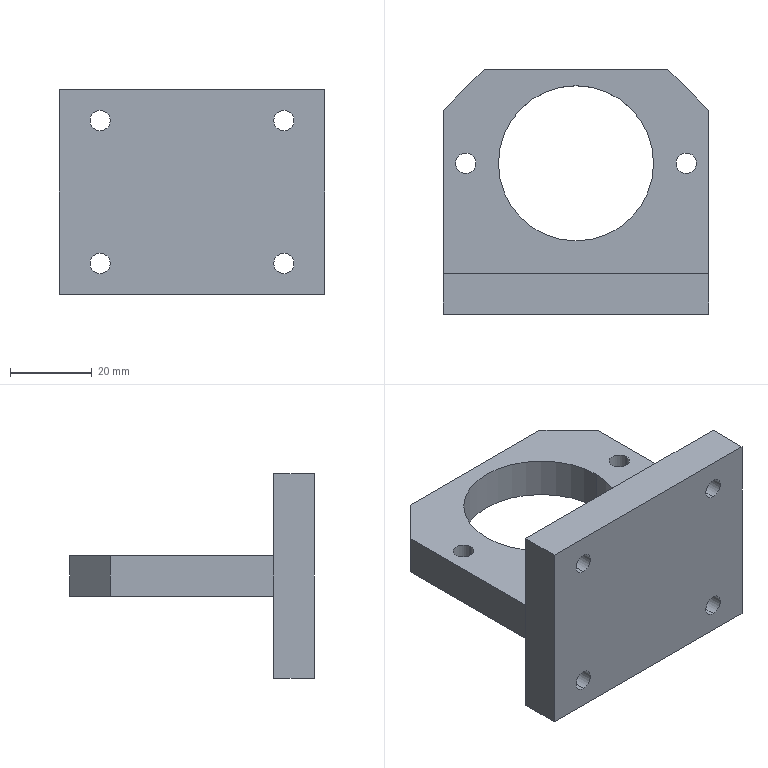Part | SolidWorks | features HoleWzd 2, ICE 2, Chamfer 1, Extrusion 1 | 2 solids | 28 faces | box 65 x 60 x 50 mm | volume 51481 mm3 | cylinder 14 | plane 14 | commonest cylinder face diameters 5 x12 38 x2
STEP:
#1=CARTESIAN_POINT('',(22.5,0.,15.));
#2=VERTEX_POINT('',#1);
#3=CARTESIAN_POINT('',(22.5,0.,20.));
#4=VERTEX_POINT('',#3);
#5=CARTESIAN_POINT('',(22.5,0.,17.5));
#6=DIRECTION('',(0.,1.,0.));
#7=DIRECTION('',(0.,0.,1.));
#8=AXIS2_PLACEMENT_3D('',#5,#6,#7);
#9=CIRCLE('',#8,2.5);
#10=EDGE_CURVE('',#2,#4,#9,.T.);
#11=ORIENTED_EDGE('',*,*,#10,.F.);
#12=CARTESIAN_POINT('',(22.5,10.,15.));
#13=VERTEX_POINT('',#12);
#14=CARTESIAN_POINT('',(22.5,10.,15.));
#15=DIRECTION('',(0.,1.,0.));
#16=VECTOR('',#15,1000.);
#17=LINE('',#14,#16);
#18=EDGE_CURVE('',#2,#13,#17,.T.);
#19=ORIENTED_EDGE('',*,*,#18,.T.);
#20=CARTESIAN_POINT('',(22.5,10.,20.));
#21=VERTEX_POINT('',#20);
#22=CARTESIAN_POINT('',(22.5,10.,17.5));
#23=DIRECTION('',(0.,1.,0.));
#24=DIRECTION('',(0.,0.,1.));
#25=AXIS2_PLACEMENT_3D('',#22,#23,#24);
#26=CIRCLE('',#25,2.5);
#27=EDGE_CURVE('',#13,#21,#26,.T.);
#28=ORIENTED_EDGE('',*,*,#27,.T.);
#29=CARTESIAN_POINT('',(22.5,10.,20.));
#30=DIRECTION('',(0.,1.,0.));
#31=VECTOR('',#30,1000.);
#32=LINE('',#29,#31);
#33=EDGE_CURVE('',#4,#21,#32,.T.);
#34=ORIENTED_EDGE('',*,*,#33,.F.);
#35=EDGE_LOOP('',(#11,#19,#28,#34));
#36=FACE_OUTER_BOUND('',#35,.T.);
#37=CARTESIAN_POINT('',(22.5,10.,17.5));
#38=DIRECTION('',(0.,1.,0.));
#39=DIRECTION('',(0.,0.,1.));
#40=AXIS2_PLACEMENT_3D('',#37,#38,#39);
#41=CYLINDRICAL_SURFACE('',#40,2.5);
#42=ADVANCED_FACE('',(#36),#41,.F.);
#43=CARTESIAN_POINT('',(-22.5,0.,-20.));
#44=VERTEX_POINT('',#43);
#45=CARTESIAN_POINT('',(-22.5,0.,-15.));
#46=VERTEX_POINT('',#45);
#47=CARTESIAN_POINT('',(-22.5,0.,-17.5));
#48=DIRECTION('',(0.,1.,0.));
#49=DIRECTION('',(0.,0.,1.));
#50=AXIS2_PLACEMENT_3D('',#47,#48,#49);
#51=CIRCLE('',#50,2.5);
#52=EDGE_CURVE('',#44,#46,#51,.T.);
#53=ORIENTED_EDGE('',*,*,#52,.F.);
#54=CARTESIAN_POINT('',(-22.5,10.,-20.));
#55=VERTEX_POINT('',#54);
#56=CARTESIAN_POINT('',(-22.5,10.,-20.));
#57=DIRECTION('',(0.,1.,0.));
#58=VECTOR('',#57,1000.);
#59=LINE('',#56,#58);
#60=EDGE_CURVE('',#44,#55,#59,.T.);
#61=ORIENTED_EDGE('',*,*,#60,.T.);
#62=CARTESIAN_POINT('',(-22.5,10.,-15.));
#63=VERTEX_POINT('',#62);
#64=CARTESIAN_POINT('',(-22.5,10.,-17.5));
#65=DIRECTION('',(0.,1.,0.));
#66=DIRECTION('',(0.,0.,1.));
#67=AXIS2_PLACEMENT_3D('',#64,#65,#66);
#68=CIRCLE('',#67,2.5);
#69=EDGE_CURVE('',#55,#63,#68,.T.);
#70=ORIENTED_EDGE('',*,*,#69,.T.);
#71=CARTESIAN_POINT('',(-22.5,10.,-15.));
#72=DIRECTION('',(0.,1.,0.));
#73=VECTOR('',#72,1000.);
#74=LINE('',#71,#73);
#75=EDGE_CURVE('',#46,#63,#74,.T.);
#76=ORIENTED_EDGE('',*,*,#75,.F.);
#77=EDGE_LOOP('',(#53,#61,#70,#76));
#78=FACE_OUTER_BOUND('',#77,.T.);
#79=CARTESIAN_POINT('',(-22.5,10.,-17.5));
#80=DIRECTION('',(0.,1.,0.));
#81=DIRECTION('',(0.,0.,1.));
#82=AXIS2_PLACEMENT_3D('',#79,#80,#81);
#83=CYLINDRICAL_SURFACE('',#82,2.5);
#84=ADVANCED_FACE('',(#78),#83,.F.);
#85=CARTESIAN_POINT('',(-22.5,0.,15.));
#86=VERTEX_POINT('',#85);
#87=CARTESIAN_POINT('',(-22.5,0.,20.));
#88=VERTEX_POINT('',#87);
#89=CARTESIAN_POINT('',(-22.5,0.,17.5));
#90=DIRECTION('',(0.,1.,0.));
#91=DIRECTION('',(0.,0.,1.));
#92=AXIS2_PLACEMENT_3D('',#89,#90,#91);
#93=CIRCLE('',#92,2.5);
#94=EDGE_CURVE('',#86,#88,#93,.T.);
#95=ORIENTED_EDGE('',*,*,#94,.F.);
#96=CARTESIAN_POINT('',(-22.5,10.,15.));
#97=VERTEX_POINT('',#96);
#98=CARTESIAN_POINT('',(-22.5,10.,15.));
#99=DIRECTION('',(0.,1.,0.));
#100=VECTOR('',#99,1000.);
#101=LINE('',#98,#100);
#102=EDGE_CURVE('',#86,#97,#101,.T.);
#103=ORIENTED_EDGE('',*,*,#102,.T.);
#104=CARTESIAN_POINT('',(-22.5,10.,20.));
#105=VERTEX_POINT('',#104);
#106=CARTESIAN_POINT('',(-22.5,10.,17.5));
#107=DIRECTION('',(0.,1.,0.));
#108=DIRECTION('',(0.,0.,1.));
#109=AXIS2_PLACEMENT_3D('',#106,#107,#108);
#110=CIRCLE('',#109,2.5);
#111=EDGE_CURVE('',#97,#105,#110,.T.);
#112=ORIENTED_EDGE('',*,*,#111,.T.);
#113=CARTESIAN_POINT('',(-22.5,10.,20.));
#114=DIRECTION('',(0.,1.,0.));
#115=VECTOR('',#114,1000.);
#116=LINE('',#113,#115);
#117=EDGE_CURVE('',#88,#105,#116,.T.);
#118=ORIENTED_EDGE('',*,*,#117,.F.);
#119=EDGE_LOOP('',(#95,#103,#112,#118));
#120=FACE_OUTER_BOUND('',#119,.T.);
#121=CARTESIAN_POINT('',(-22.5,10.,17.5));
#122=DIRECTION('',(0.,1.,0.));
#123=DIRECTION('',(0.,0.,1.));
#124=AXIS2_PLACEMENT_3D('',#121,#122,#123);
#125=CYLINDRICAL_SURFACE('',#124,2.5);
#126=ADVANCED_FACE('',(#120),#125,.F.);
#127=CARTESIAN_POINT('',(22.5,0.,-20.));
#128=VERTEX_POINT('',#127);
#129=CARTESIAN_POINT('',(22.5,0.,-15.));
#130=VERTEX_POINT('',#129);
#131=CARTESIAN_POINT('',(22.5,0.,-17.5));
#132=DIRECTION('',(0.,1.,0.));
#133=DIRECTION('',(0.,0.,1.));
#134=AXIS2_PLACEMENT_3D('',#131,#132,#133);
#135=CIRCLE('',#134,2.5);
#136=EDGE_CURVE('',#128,#130,#135,.T.);
#137=ORIENTED_EDGE('',*,*,#136,.F.);
#138=CARTESIAN_POINT('',(22.5,10.,-20.));
#139=VERTEX_POINT('',#138);
#140=CARTESIAN_POINT('',(22.5,10.,-20.));
#141=DIRECTION('',(0.,1.,0.));
#142=VECTOR('',#141,1000.);
#143=LINE('',#140,#142);
#144=EDGE_CURVE('',#128,#139,#143,.T.);
#145=ORIENTED_EDGE('',*,*,#144,.T.);
#146=CARTESIAN_POINT('',(22.5,10.,-15.));
#147=VERTEX_POINT('',#146);
#148=CARTESIAN_POINT('',(22.5,10.,-17.5));
#149=DIRECTION('',(0.,1.,0.));
#150=DIRECTION('',(0.,0.,1.));
#151=AXIS2_PLACEMENT_3D('',#148,#149,#150);
#152=CIRCLE('',#151,2.5);
#153=EDGE_CURVE('',#139,#147,#152,.T.);
#154=ORIENTED_EDGE('',*,*,#153,.T.);
#155=CARTESIAN_POINT('',(22.5,10.,-15.));
#156=DIRECTION('',(0.,1.,0.));
#157=VECTOR('',#156,1000.);
#158=LINE('',#155,#157);
#159=EDGE_CURVE('',#130,#147,#158,.T.);
#160=ORIENTED_EDGE('',*,*,#159,.F.);
#161=EDGE_LOOP('',(#137,#145,#154,#160));
#162=FACE_OUTER_BOUND('',#161,.T.);
#163=CARTESIAN_POINT('',(22.5,10.,-17.5));
#164=DIRECTION('',(0.,1.,0.));
#165=DIRECTION('',(0.,0.,1.));
#166=AXIS2_PLACEMENT_3D('',#163,#164,#165);
#167=CYLINDRICAL_SURFACE('',#166,2.5);
#168=ADVANCED_FACE('',(#162),#167,.F.);
#169=CARTESIAN_POINT('',(32.5,0.,25.));
#170=VERTEX_POINT('',#169);
#171=CARTESIAN_POINT('',(32.5,0.,-25.));
#172=VERTEX_POINT('',#171);
#173=CARTESIAN_POINT('',(32.5,0.,-25.));
#174=DIRECTION('',(0.,0.,-1.));
#175=VECTOR('',#174,1000.);
#176=LINE('',#173,#175);
#177=EDGE_CURVE('',#170,#172,#176,.T.);
#178=ORIENTED_EDGE('',*,*,#177,.T.);
#179=CARTESIAN_POINT('',(32.5,10.,-25.));
#180=VERTEX_POINT('',#179);
#181=CARTESIAN_POINT('',(32.5,10.,-25.));
#182=DIRECTION('',(0.,-1.,0.));
#183=VECTOR('',#182,1000.);
#184=LINE('',#181,#183);
#185=EDGE_CURVE('',#180,#172,#184,.T.);
#186=ORIENTED_EDGE('',*,*,#185,.F.);
#187=CARTESIAN_POINT('',(32.5,10.,25.));
#188=VERTEX_POINT('',#187);
#189=CARTESIAN_POINT('',(32.5,10.,-25.));
#190=DIRECTION('',(0.,0.,-1.));
#191=VECTOR('',#190,1000.);
#192=LINE('',#189,#191);
#193=EDGE_CURVE('',#188,#180,#192,.T.);
#194=ORIENTED_EDGE('',*,*,#193,.F.);
#195=CARTESIAN_POINT('',(32.5,10.,25.));
#196=DIRECTION('',(0.,-1.,0.));
#197=VECTOR('',#196,1000.);
#198=LINE('',#195,#197);
#199=EDGE_CURVE('',#188,#170,#198,.T.);
#200=ORIENTED_EDGE('',*,*,#199,.T.);
#201=EDGE_LOOP('',(#178,#186,#194,#200));
#202=FACE_OUTER_BOUND('',#201,.T.);
#203=CARTESIAN_POINT('',(32.5,10.,-25.));
#204=DIRECTION('',(-1.,0.,0.));
#205=DIRECTION('',(0.,0.,1.));
#206=AXIS2_PLACEMENT_3D('',#203,#204,#205);
#207=PLANE('',#206);
#208=ADVANCED_FACE('',(#202),#207,.F.);
#209=CARTESIAN_POINT('',(-32.5,0.,-25.));
#210=VERTEX_POINT('',#209);
#211=CARTESIAN_POINT('',(-32.5,0.,-25.));
#212=DIRECTION('',(-1.,0.,0.));
#213=VECTOR('',#212,1000.);
#214=LINE('',#211,#213);
#215=EDGE_CURVE('',#172,#210,#214,.T.);
#216=ORIENTED_EDGE('',*,*,#215,.T.);
#217=CARTESIAN_POINT('',(-32.5,10.,-25.));
#218=VERTEX_POINT('',#217);
#219=CARTESIAN_POINT('',(-32.5,10.,-25.));
#220=DIRECTION('',(0.,-1.,0.));
#221=VECTOR('',#220,1000.);
#222=LINE('',#219,#221);
#223=EDGE_CURVE('',#218,#210,#222,.T.);
#224=ORIENTED_EDGE('',*,*,#223,.F.);
#225=CARTESIAN_POINT('',(-32.5,10.,-25.));
#226=DIRECTION('',(-1.,0.,0.));
#227=VECTOR('',#226,1000.);
#228=LINE('',#225,#227);
#229=EDGE_CURVE('',#180,#218,#228,.T.);
#230=ORIENTED_EDGE('',*,*,#229,.F.);
#231=ORIENTED_EDGE('',*,*,#185,.T.);
#232=EDGE_LOOP('',(#216,#224,#230,#231));
#233=FACE_OUTER_BOUND('',#232,.T.);
#234=CARTESIAN_POINT('',(-32.5,10.,-25.));
#235=DIRECTION('',(0.,0.,1.));
#236=DIRECTION('',(1.,0.,0.));
#237=AXIS2_PLACEMENT_3D('',#234,#235,#236);
#238=PLANE('',#237);
#239=ADVANCED_FACE('',(#233),#238,.F.);
#240=CARTESIAN_POINT('',(-32.5,0.,25.));
#241=VERTEX_POINT('',#240);
#242=CARTESIAN_POINT('',(-32.5,0.,-25.));
#243=DIRECTION('',(0.,0.,1.));
#244=VECTOR('',#243,1000.);
#245=LINE('',#242,#244);
#246=EDGE_CURVE('',#210,#241,#245,.T.);
#247=ORIENTED_EDGE('',*,*,#246,.T.);
#248=CARTESIAN_POINT('',(-32.5,10.,25.));
#249=VERTEX_POINT('',#248);
#250=CARTESIAN_POINT('',(-32.5,10.,25.));
#251=DIRECTION('',(0.,-1.,0.));
#252=VECTOR('',#251,1000.);
#253=LINE('',#250,#252);
#254=EDGE_CURVE('',#249,#241,#253,.T.);
#255=ORIENTED_EDGE('',*,*,#254,.F.);
#256=CARTESIAN_POINT('',(-32.5,10.,-25.));
#257=DIRECTION('',(0.,0.,1.));
#258=VECTOR('',#257,1000.);
#259=LINE('',#256,#258);
#260=EDGE_CURVE('',#218,#249,#259,.T.);
#261=ORIENTED_EDGE('',*,*,#260,.F.);
#262=ORIENTED_EDGE('',*,*,#223,.T.);
#263=EDGE_LOOP('',(#247,#255,#261,#262));
#264=FACE_OUTER_BOUND('',#263,.T.);
#265=CARTESIAN_POINT('',(-32.5,10.,-25.));
#266=DIRECTION('',(1.,0.,0.));
#267=DIRECTION('',(0.,0.,-1.));
#268=AXIS2_PLACEMENT_3D('',#265,#266,#267);
#269=PLANE('',#268);
#270=ADVANCED_FACE('',(#264),#269,.F.);
#271=CARTESIAN_POINT('',(-32.5,0.,25.));
#272=DIRECTION('',(1.,0.,0.));
#273=VECTOR('',#272,1000.);
#274=LINE('',#271,#273);
#275=EDGE_CURVE('',#241,#170,#274,.T.);
#276=ORIENTED_EDGE('',*,*,#275,.T.);
#277=ORIENTED_EDGE('',*,*,#199,.F.);
#278=CARTESIAN_POINT('',(-32.5,10.,25.));
#279=DIRECTION('',(1.,0.,0.));
#280=VECTOR('',#279,1000.);
#281=LINE('',#278,#280);
#282=EDGE_CURVE('',#249,#188,#281,.T.);
#283=ORIENTED_EDGE('',*,*,#282,.F.);
#284=ORIENTED_EDGE('',*,*,#254,.T.);
#285=EDGE_LOOP('',(#276,#277,#283,#284));
#286=FACE_OUTER_BOUND('',#285,.T.);
#287=CARTESIAN_POINT('',(-32.5,10.,25.));
#288=DIRECTION('',(0.,0.,-1.));
#289=DIRECTION('',(-1.,0.,0.));
#290=AXIS2_PLACEMENT_3D('',#287,#288,#289);
#291=PLANE('',#290);
#292=ADVANCED_FACE('',(#286),#291,.F.);
#293=CARTESIAN_POINT('',(22.5,10.,17.5));
#294=DIRECTION('',(0.,1.,0.));
#295=DIRECTION('',(0.,0.,1.));
#296=AXIS2_PLACEMENT_3D('',#293,#294,#295);
#297=CIRCLE('',#296,2.5);
#298=EDGE_CURVE('',#21,#13,#297,.T.);
#299=ORIENTED_EDGE('',*,*,#298,.F.);
#300=ORIENTED_EDGE('',*,*,#27,.F.);
#301=EDGE_LOOP('',(#299,#300));
#302=FACE_BOUND('',#301,.T.);
#303=CARTESIAN_POINT('',(-22.5,10.,-17.5));
#304=DIRECTION('',(0.,1.,0.));
#305=DIRECTION('',(0.,0.,1.));
#306=AXIS2_PLACEMENT_3D('',#303,#304,#305);
#307=CIRCLE('',#306,2.5);
#308=EDGE_CURVE('',#63,#55,#307,.T.);
#309=ORIENTED_EDGE('',*,*,#308,.F.);
#310=ORIENTED_EDGE('',*,*,#69,.F.);
#311=EDGE_LOOP('',(#309,#310));
#312=FACE_BOUND('',#311,.T.);
#313=CARTESIAN_POINT('',(-22.5,10.,17.5));
#314=DIRECTION('',(0.,1.,0.));
#315=DIRECTION('',(0.,0.,1.));
#316=AXIS2_PLACEMENT_3D('',#313,#314,#315);
#317=CIRCLE('',#316,2.5);
#318=EDGE_CURVE('',#105,#97,#317,.T.);
#319=ORIENTED_EDGE('',*,*,#318,.F.);
#320=ORIENTED_EDGE('',*,*,#111,.F.);
#321=EDGE_LOOP('',(#319,#320));
#322=FACE_BOUND('',#321,.T.);
#323=CARTESIAN_POINT('',(22.5,10.,-17.5));
#324=DIRECTION('',(0.,1.,0.));
#325=DIRECTION('',(0.,0.,1.));
#326=AXIS2_PLACEMENT_3D('',#323,#324,#325);
#327=CIRCLE('',#326,2.5);
#328=EDGE_CURVE('',#147,#139,#327,.T.);
#329=ORIENTED_EDGE('',*,*,#328,.F.);
#330=ORIENTED_EDGE('',*,*,#153,.F.);
#331=EDGE_LOOP('',(#329,#330));
#332=FACE_BOUND('',#331,.T.);
#333=ORIENTED_EDGE('',*,*,#193,.T.);
#334=ORIENTED_EDGE('',*,*,#229,.T.);
#335=ORIENTED_EDGE('',*,*,#260,.T.);
#336=ORIENTED_EDGE('',*,*,#282,.T.);
#337=EDGE_LOOP('',(#333,#334,#335,#336));
#338=FACE_OUTER_BOUND('',#337,.T.);
#339=CARTESIAN_POINT('',(0.,10.,0.));
#340=DIRECTION('',(0.,1.,0.));
#341=DIRECTION('',(0.,0.,1.));
#342=AXIS2_PLACEMENT_3D('',#339,#340,#341);
#343=PLANE('',#342);
#344=ADVANCED_FACE('',(#302,#312,#322,#332,#338),#343,.T.);
#345=CARTESIAN_POINT('',(22.5,0.,17.5));
#346=DIRECTION('',(0.,1.,0.));
#347=DIRECTION('',(0.,0.,1.));
#348=AXIS2_PLACEMENT_3D('',#345,#346,#347);
#349=CIRCLE('',#348,2.5);
#350=EDGE_CURVE('',#4,#2,#349,.T.);
#351=ORIENTED_EDGE('',*,*,#350,.T.);
#352=ORIENTED_EDGE('',*,*,#10,.T.);
#353=EDGE_LOOP('',(#351,#352));
#354=FACE_BOUND('',#353,.T.);
#355=CARTESIAN_POINT('',(-22.5,0.,-17.5));
#356=DIRECTION('',(0.,1.,0.));
#357=DIRECTION('',(0.,0.,1.));
#358=AXIS2_PLACEMENT_3D('',#355,#356,#357);
#359=CIRCLE('',#358,2.5);
#360=EDGE_CURVE('',#46,#44,#359,.T.);
#361=ORIENTED_EDGE('',*,*,#360,.T.);
#362=ORIENTED_EDGE('',*,*,#52,.T.);
#363=EDGE_LOOP('',(#361,#362));
#364=FACE_BOUND('',#363,.T.);
#365=CARTESIAN_POINT('',(-22.5,0.,17.5));
#366=DIRECTION('',(0.,1.,0.));
#367=DIRECTION('',(0.,0.,1.));
#368=AXIS2_PLACEMENT_3D('',#365,#366,#367);
#369=CIRCLE('',#368,2.5);
#370=EDGE_CURVE('',#88,#86,#369,.T.);
#371=ORIENTED_EDGE('',*,*,#370,.T.);
#372=ORIENTED_EDGE('',*,*,#94,.T.);
#373=EDGE_LOOP('',(#371,#372));
#374=FACE_BOUND('',#373,.T.);
#375=CARTESIAN_POINT('',(22.5,0.,-17.5));
#376=DIRECTION('',(0.,1.,0.));
#377=DIRECTION('',(0.,0.,1.));
#378=AXIS2_PLACEMENT_3D('',#375,#376,#377);
#379=CIRCLE('',#378,2.5);
#380=EDGE_CURVE('',#130,#128,#379,.T.);
#381=ORIENTED_EDGE('',*,*,#380,.T.);
#382=ORIENTED_EDGE('',*,*,#136,.T.);
#383=EDGE_LOOP('',(#381,#382));
#384=FACE_BOUND('',#383,.T.);
#385=ORIENTED_EDGE('',*,*,#177,.F.);
#386=ORIENTED_EDGE('',*,*,#275,.F.);
#387=ORIENTED_EDGE('',*,*,#246,.F.);
#388=ORIENTED_EDGE('',*,*,#215,.F.);
#389=EDGE_LOOP('',(#385,#386,#387,#388));
#390=FACE_OUTER_BOUND('',#389,.T.);
#391=CARTESIAN_POINT('',(0.,0.,0.));
#392=DIRECTION('',(0.,1.,0.));
#393=DIRECTION('',(0.,0.,1.));
#394=AXIS2_PLACEMENT_3D('',#391,#392,#393);
#395=PLANE('',#394);
#396=ADVANCED_FACE('',(#354,#364,#374,#384,#390),#395,.F.);
#397=ORIENTED_EDGE('',*,*,#144,.F.);
#398=ORIENTED_EDGE('',*,*,#380,.F.);
#399=ORIENTED_EDGE('',*,*,#159,.T.);
#400=ORIENTED_EDGE('',*,*,#328,.T.);
#401=EDGE_LOOP('',(#397,#398,#399,#400));
#402=FACE_OUTER_BOUND('',#401,.T.);
#403=CARTESIAN_POINT('',(22.5,10.,-17.5));
#404=DIRECTION('',(0.,1.,0.));
#405=DIRECTION('',(0.,0.,1.));
#406=AXIS2_PLACEMENT_3D('',#403,#404,#405);
#407=CYLINDRICAL_SURFACE('',#406,2.5);
#408=ADVANCED_FACE('',(#402),#407,.F.);
#409=ORIENTED_EDGE('',*,*,#102,.F.);
#410=ORIENTED_EDGE('',*,*,#370,.F.);
#411=ORIENTED_EDGE('',*,*,#117,.T.);
#412=ORIENTED_EDGE('',*,*,#318,.T.);
#413=EDGE_LOOP('',(#409,#410,#411,#412));
#414=FACE_OUTER_BOUND('',#413,.T.);
#415=CARTESIAN_POINT('',(-22.5,10.,17.5));
#416=DIRECTION('',(0.,1.,0.));
#417=DIRECTION('',(0.,0.,1.));
#418=AXIS2_PLACEMENT_3D('',#415,#416,#417);
#419=CYLINDRICAL_SURFACE('',#418,2.5);
#420=ADVANCED_FACE('',(#414),#419,.F.);
#421=ORIENTED_EDGE('',*,*,#60,.F.);
#422=ORIENTED_EDGE('',*,*,#360,.F.);
#423=ORIENTED_EDGE('',*,*,#75,.T.);
#424=ORIENTED_EDGE('',*,*,#308,.T.);
#425=EDGE_LOOP('',(#421,#422,#423,#424));
#426=FACE_OUTER_BOUND('',#425,.T.);
#427=CARTESIAN_POINT('',(-22.5,10.,-17.5));
#428=DIRECTION('',(0.,1.,0.));
#429=DIRECTION('',(0.,0.,1.));
#430=AXIS2_PLACEMENT_3D('',#427,#428,#429);
#431=CYLINDRICAL_SURFACE('',#430,2.5);
#432=ADVANCED_FACE('',(#426),#431,.F.);
#433=ORIENTED_EDGE('',*,*,#18,.F.);
#434=ORIENTED_EDGE('',*,*,#350,.F.);
#435=ORIENTED_EDGE('',*,*,#33,.T.);
#436=ORIENTED_EDGE('',*,*,#298,.T.);
#437=EDGE_LOOP('',(#433,#434,#435,#436));
#438=FACE_OUTER_BOUND('',#437,.T.);
#439=CARTESIAN_POINT('',(22.5,10.,17.5));
#440=DIRECTION('',(0.,1.,0.));
#441=DIRECTION('',(0.,0.,1.));
#442=AXIS2_PLACEMENT_3D('',#439,#440,#441);
#443=CYLINDRICAL_SURFACE('',#442,2.5);
#444=ADVANCED_FACE('',(#438),#443,.F.);
#445=CLOSED_SHELL('',(#42,#84,#126,#168,#208,#239,#270,#292,#344,#396,#408,#420,#432,#444));
#446=MANIFOLD_SOLID_BREP('',#445);
#447=CARTESIAN_POINT('',(-29.5,37.,-5.));
#448=VERTEX_POINT('',#447);
#449=CARTESIAN_POINT('',(-24.5,37.,-5.));
#450=VERTEX_POINT('',#449);
#451=CARTESIAN_POINT('',(-27.,37.,-5.));
#452=DIRECTION('',(0.,0.,1.));
#453=DIRECTION('',(1.,0.,0.));
#454=AXIS2_PLACEMENT_3D('',#451,#452,#453);
#455=CIRCLE('',#454,2.5);
#456=EDGE_CURVE('',#448,#450,#455,.T.);
#457=ORIENTED_EDGE('',*,*,#456,.F.);
#458=CARTESIAN_POINT('',(-29.5,37.,5.));
#459=VERTEX_POINT('',#458);
#460=CARTESIAN_POINT('',(-29.5,37.,5.));
#461=DIRECTION('',(0.,0.,1.));
#462=VECTOR('',#461,1000.);
#463=LINE('',#460,#462);
#464=EDGE_CURVE('',#448,#459,#463,.T.);
#465=ORIENTED_EDGE('',*,*,#464,.T.);
#466=CARTESIAN_POINT('',(-24.5,37.,5.));
#467=VERTEX_POINT('',#466);
#468=CARTESIAN_POINT('',(-27.,37.,5.));
#469=DIRECTION('',(0.,0.,1.));
#470=DIRECTION('',(1.,0.,0.));
#471=AXIS2_PLACEMENT_3D('',#468,#469,#470);
#472=CIRCLE('',#471,2.5);
#473=EDGE_CURVE('',#459,#467,#472,.T.);
#474=ORIENTED_EDGE('',*,*,#473,.T.);
#475=CARTESIAN_POINT('',(-24.5,37.,5.));
#476=DIRECTION('',(0.,0.,1.));
#477=VECTOR('',#476,1000.);
#478=LINE('',#475,#477);
#479=EDGE_CURVE('',#450,#467,#478,.T.);
#480=ORIENTED_EDGE('',*,*,#479,.F.);
#481=EDGE_LOOP('',(#457,#465,#474,#480));
#482=FACE_OUTER_BOUND('',#481,.T.);
#483=CARTESIAN_POINT('',(-27.,37.,5.));
#484=DIRECTION('',(0.,0.,1.));
#485=DIRECTION('',(1.,0.,0.));
#486=AXIS2_PLACEMENT_3D('',#483,#484,#485);
#487=CYLINDRICAL_SURFACE('',#486,2.5);
#488=ADVANCED_FACE('',(#482),#487,.F.);
#489=CARTESIAN_POINT('',(24.5,37.,-5.));
#490=VERTEX_POINT('',#489);
#491=CARTESIAN_POINT('',(29.5,37.,-5.));
#492=VERTEX_POINT('',#491);
#493=CARTESIAN_POINT('',(27.,37.,-5.));
#494=DIRECTION('',(0.,0.,1.));
#495=DIRECTION('',(1.,0.,0.));
#496=AXIS2_PLACEMENT_3D('',#493,#494,#495);
#497=CIRCLE('',#496,2.5);
#498=EDGE_CURVE('',#490,#492,#497,.T.);
#499=ORIENTED_EDGE('',*,*,#498,.F.);
#500=CARTESIAN_POINT('',(24.5,37.,5.));
#501=VERTEX_POINT('',#500);
#502=CARTESIAN_POINT('',(24.5,37.,5.));
#503=DIRECTION('',(0.,0.,1.));
#504=VECTOR('',#503,1000.);
#505=LINE('',#502,#504);
#506=EDGE_CURVE('',#490,#501,#505,.T.);
#507=ORIENTED_EDGE('',*,*,#506,.T.);
#508=CARTESIAN_POINT('',(29.5,37.,5.));
#509=VERTEX_POINT('',#508);
#510=CARTESIAN_POINT('',(27.,37.,5.));
#511=DIRECTION('',(0.,0.,1.));
#512=DIRECTION('',(1.,0.,0.));
#513=AXIS2_PLACEMENT_3D('',#510,#511,#512);
#514=CIRCLE('',#513,2.5);
#515=EDGE_CURVE('',#501,#509,#514,.T.);
#516=ORIENTED_EDGE('',*,*,#515,.T.);
#517=CARTESIAN_POINT('',(29.5,37.,5.));
#518=DIRECTION('',(0.,0.,1.));
#519=VECTOR('',#518,1000.);
#520=LINE('',#517,#519);
#521=EDGE_CURVE('',#492,#509,#520,.T.);
#522=ORIENTED_EDGE('',*,*,#521,.F.);
#523=EDGE_LOOP('',(#499,#507,#516,#522));
#524=FACE_OUTER_BOUND('',#523,.T.);
#525=CARTESIAN_POINT('',(27.,37.,5.));
#526=DIRECTION('',(0.,0.,1.));
#527=DIRECTION('',(1.,0.,0.));
#528=AXIS2_PLACEMENT_3D('',#525,#526,#527);
#529=CYLINDRICAL_SURFACE('',#528,2.5);
#530=ADVANCED_FACE('',(#524),#529,.F.);
#531=CARTESIAN_POINT('',(19.,37.,-5.));
#532=VERTEX_POINT('',#531);
#533=CARTESIAN_POINT('',(-19.,37.,-5.));
#534=VERTEX_POINT('',#533);
#535=CARTESIAN_POINT('',(0.,37.,-5.));
#536=DIRECTION('',(0.,0.,-1.));
#537=DIRECTION('',(1.,0.,0.));
#538=AXIS2_PLACEMENT_3D('',#535,#536,#537);
#539=CIRCLE('',#538,19.);
#540=EDGE_CURVE('',#532,#534,#539,.T.);
#541=ORIENTED_EDGE('',*,*,#540,.T.);
#542=CARTESIAN_POINT('',(-19.,37.,5.));
#543=VERTEX_POINT('',#542);
#544=CARTESIAN_POINT('',(-19.,37.,-25.001));
#545=DIRECTION('',(0.,0.,1.));
#546=VECTOR('',#545,1000.);
#547=LINE('',#544,#546);
#548=EDGE_CURVE('',#534,#543,#547,.T.);
#549=ORIENTED_EDGE('',*,*,#548,.T.);
#550=CARTESIAN_POINT('',(19.,37.,5.));
#551=VERTEX_POINT('',#550);
#552=CARTESIAN_POINT('',(0.,37.,5.));
#553=DIRECTION('',(0.,0.,1.));
#554=DIRECTION('',(1.,0.,0.));
#555=AXIS2_PLACEMENT_3D('',#552,#553,#554);
#556=CIRCLE('',#555,19.);
#557=EDGE_CURVE('',#543,#551,#556,.T.);
#558=ORIENTED_EDGE('',*,*,#557,.T.);
#559=CARTESIAN_POINT('',(19.,37.,-25.001));
#560=DIRECTION('',(0.,0.,1.));
#561=VECTOR('',#560,1000.);
#562=LINE('',#559,#561);
#563=EDGE_CURVE('',#532,#551,#562,.T.);
#564=ORIENTED_EDGE('',*,*,#563,.F.);
#565=EDGE_LOOP('',(#541,#549,#558,#564));
#566=FACE_OUTER_BOUND('',#565,.T.);
#567=CARTESIAN_POINT('',(0.,37.,-25.001));
#568=DIRECTION('',(0.,0.,1.));
#569=DIRECTION('',(1.,0.,0.));
#570=AXIS2_PLACEMENT_3D('',#567,#568,#569);
#571=CYLINDRICAL_SURFACE('',#570,19.);
#572=ADVANCED_FACE('',(#566),#571,.F.);
#573=CARTESIAN_POINT('',(27.,37.,5.));
#574=DIRECTION('',(0.,0.,1.));
#575=DIRECTION('',(1.,0.,0.));
#576=AXIS2_PLACEMENT_3D('',#573,#574,#575);
#577=CIRCLE('',#576,2.5);
#578=EDGE_CURVE('',#509,#501,#577,.T.);
#579=ORIENTED_EDGE('',*,*,#578,.F.);
#580=ORIENTED_EDGE('',*,*,#515,.F.);
#581=EDGE_LOOP('',(#579,#580));
#582=FACE_BOUND('',#581,.T.);
#583=CARTESIAN_POINT('',(0.,37.,5.));
#584=DIRECTION('',(0.,0.,1.));
#585=DIRECTION('',(1.,0.,0.));
#586=AXIS2_PLACEMENT_3D('',#583,#584,#585);
#587=CIRCLE('',#586,19.);
#588=EDGE_CURVE('',#551,#543,#587,.T.);
#589=ORIENTED_EDGE('',*,*,#588,.F.);
#590=ORIENTED_EDGE('',*,*,#557,.F.);
#591=EDGE_LOOP('',(#589,#590));
#592=FACE_BOUND('',#591,.T.);
#593=CARTESIAN_POINT('',(32.5,50.,5.));
#594=VERTEX_POINT('',#593);
#595=CARTESIAN_POINT('',(32.5,10.,5.));
#596=VERTEX_POINT('',#595);
#597=CARTESIAN_POINT('',(32.5,60.,5.));
#598=DIRECTION('',(0.,-1.,0.));
#599=VECTOR('',#598,1000.);
#600=LINE('',#597,#599);
#601=EDGE_CURVE('',#594,#596,#600,.T.);
#602=ORIENTED_EDGE('',*,*,#601,.F.);
#603=CARTESIAN_POINT('',(22.5,60.,5.));
#604=VERTEX_POINT('',#603);
#605=CARTESIAN_POINT('',(22.5,60.,5.));
#606=DIRECTION('',(-0.7071,0.7071,0.));
#607=VECTOR('',#606,1000.);
#608=LINE('',#605,#607);
#609=EDGE_CURVE('',#594,#604,#608,.T.);
#610=ORIENTED_EDGE('',*,*,#609,.T.);
#611=CARTESIAN_POINT('',(-22.5,60.,5.));
#612=VERTEX_POINT('',#611);
#613=CARTESIAN_POINT('',(-32.5,60.,5.));
#614=DIRECTION('',(1.,0.,0.));
#615=VECTOR('',#614,1000.);
#616=LINE('',#613,#615);
#617=EDGE_CURVE('',#612,#604,#616,.T.);
#618=ORIENTED_EDGE('',*,*,#617,.F.);
#619=CARTESIAN_POINT('',(-32.5,50.,5.));
#620=VERTEX_POINT('',#619);
#621=CARTESIAN_POINT('',(-22.5,60.,5.));
#622=DIRECTION('',(-0.7071,-0.7071,0.));
#623=VECTOR('',#622,1000.);
#624=LINE('',#621,#623);
#625=EDGE_CURVE('',#612,#620,#624,.T.);
#626=ORIENTED_EDGE('',*,*,#625,.T.);
#627=CARTESIAN_POINT('',(-32.5,10.,5.));
#628=VERTEX_POINT('',#627);
#629=CARTESIAN_POINT('',(-32.5,60.,5.));
#630=DIRECTION('',(0.,-1.,0.));
#631=VECTOR('',#630,1000.);
#632=LINE('',#629,#631);
#633=EDGE_CURVE('',#620,#628,#632,.T.);
#634=ORIENTED_EDGE('',*,*,#633,.T.);
#635=CARTESIAN_POINT('',(-32.5,10.,5.));
#636=DIRECTION('',(1.,0.,0.));
#637=VECTOR('',#636,1000.);
#638=LINE('',#635,#637);
#639=EDGE_CURVE('',#628,#596,#638,.T.);
#640=ORIENTED_EDGE('',*,*,#639,.T.);
#641=EDGE_LOOP('',(#602,#610,#618,#626,#634,#640));
#642=FACE_OUTER_BOUND('',#641,.T.);
#643=CARTESIAN_POINT('',(-27.,37.,5.));
#644=DIRECTION('',(0.,0.,1.));
#645=DIRECTION('',(1.,0.,0.));
#646=AXIS2_PLACEMENT_3D('',#643,#644,#645);
#647=CIRCLE('',#646,2.5);
#648=EDGE_CURVE('',#467,#459,#647,.T.);
#649=ORIENTED_EDGE('',*,*,#648,.F.);
#650=ORIENTED_EDGE('',*,*,#473,.F.);
#651=EDGE_LOOP('',(#649,#650));
#652=FACE_BOUND('',#651,.T.);
#653=CARTESIAN_POINT('',(-32.5,60.,5.));
#654=DIRECTION('',(0.,0.,-1.));
#655=DIRECTION('',(-1.,0.,0.));
#656=AXIS2_PLACEMENT_3D('',#653,#654,#655);
#657=PLANE('',#656);
#658=ADVANCED_FACE('',(#582,#592,#642,#652),#657,.F.);
#659=CARTESIAN_POINT('',(32.5,50.,-5.));
#660=VERTEX_POINT('',#659);
#661=CARTESIAN_POINT('',(32.5,10.,-5.));
#662=VERTEX_POINT('',#661);
#663=CARTESIAN_POINT('',(32.5,60.,-5.));
#664=DIRECTION('',(0.,-1.,0.));
#665=VECTOR('',#664,1000.);
#666=LINE('',#663,#665);
#667=EDGE_CURVE('',#660,#662,#666,.T.);
#668=ORIENTED_EDGE('',*,*,#667,.F.);
#669=CARTESIAN_POINT('',(32.5,50.,5.));
#670=DIRECTION('',(0.,0.,1.));
#671=VECTOR('',#670,1000.);
#672=LINE('',#669,#671);
#673=EDGE_CURVE('',#660,#594,#672,.T.);
#674=ORIENTED_EDGE('',*,*,#673,.T.);
#675=ORIENTED_EDGE('',*,*,#601,.T.);
#676=CARTESIAN_POINT('',(32.5,10.,-5.));
#677=DIRECTION('',(0.,0.,-1.));
#678=VECTOR('',#677,1000.);
#679=LINE('',#676,#678);
#680=EDGE_CURVE('',#596,#662,#679,.T.);
#681=ORIENTED_EDGE('',*,*,#680,.T.);
#682=EDGE_LOOP('',(#668,#674,#675,#681));
#683=FACE_OUTER_BOUND('',#682,.T.);
#684=CARTESIAN_POINT('',(32.5,60.,-5.));
#685=DIRECTION('',(-1.,0.,0.));
#686=DIRECTION('',(0.,0.,1.));
#687=AXIS2_PLACEMENT_3D('',#684,#685,#686);
#688=PLANE('',#687);
#689=ADVANCED_FACE('',(#683),#688,.F.);
#690=CARTESIAN_POINT('',(-27.,37.,-5.));
#691=DIRECTION('',(0.,0.,1.));
#692=DIRECTION('',(1.,0.,0.));
#693=AXIS2_PLACEMENT_3D('',#690,#691,#692);
#694=CIRCLE('',#693,2.5);
#695=EDGE_CURVE('',#450,#448,#694,.T.);
#696=ORIENTED_EDGE('',*,*,#695,.T.);
#697=ORIENTED_EDGE('',*,*,#456,.T.);
#698=EDGE_LOOP('',(#696,#697));
#699=FACE_BOUND('',#698,.T.);
#700=CARTESIAN_POINT('',(27.,37.,-5.));
#701=DIRECTION('',(0.,0.,1.));
#702=DIRECTION('',(1.,0.,0.));
#703=AXIS2_PLACEMENT_3D('',#700,#701,#702);
#704=CIRCLE('',#703,2.5);
#705=EDGE_CURVE('',#492,#490,#704,.T.);
#706=ORIENTED_EDGE('',*,*,#705,.T.);
#707=ORIENTED_EDGE('',*,*,#498,.T.);
#708=EDGE_LOOP('',(#706,#707));
#709=FACE_BOUND('',#708,.T.);
#710=ORIENTED_EDGE('',*,*,#540,.F.);
#711=CARTESIAN_POINT('',(0.,37.,-5.));
#712=DIRECTION('',(0.,0.,-1.));
#713=DIRECTION('',(1.,0.,0.));
#714=AXIS2_PLACEMENT_3D('',#711,#712,#713);
#715=CIRCLE('',#714,19.);
#716=EDGE_CURVE('',#534,#532,#715,.T.);
#717=ORIENTED_EDGE('',*,*,#716,.F.);
#718=EDGE_LOOP('',(#710,#717));
#719=FACE_BOUND('',#718,.T.);
#720=CARTESIAN_POINT('',(22.5,60.,-5.));
#721=VERTEX_POINT('',#720);
#722=CARTESIAN_POINT('',(-22.5,60.,-5.));
#723=VERTEX_POINT('',#722);
#724=CARTESIAN_POINT('',(-32.5,60.,-5.));
#725=DIRECTION('',(-1.,0.,0.));
#726=VECTOR('',#725,1000.);
#727=LINE('',#724,#726);
#728=EDGE_CURVE('',#721,#723,#727,.T.);
#729=ORIENTED_EDGE('',*,*,#728,.F.);
#730=CARTESIAN_POINT('',(22.5,60.,-5.));
#731=DIRECTION('',(0.7071,-0.7071,0.));
#732=VECTOR('',#731,1000.);
#733=LINE('',#730,#732);
#734=EDGE_CURVE('',#721,#660,#733,.T.);
#735=ORIENTED_EDGE('',*,*,#734,.T.);
#736=ORIENTED_EDGE('',*,*,#667,.T.);
#737=CARTESIAN_POINT('',(-32.5,10.,-5.));
#738=VERTEX_POINT('',#737);
#739=CARTESIAN_POINT('',(-32.5,10.,-5.));
#740=DIRECTION('',(-1.,0.,0.));
#741=VECTOR('',#740,1000.);
#742=LINE('',#739,#741);
#743=EDGE_CURVE('',#662,#738,#742,.T.);
#744=ORIENTED_EDGE('',*,*,#743,.T.);
#745=CARTESIAN_POINT('',(-32.5,50.,-5.));
#746=VERTEX_POINT('',#745);
#747=CARTESIAN_POINT('',(-32.5,60.,-5.));
#748=DIRECTION('',(0.,-1.,0.));
#749=VECTOR('',#748,1000.);
#750=LINE('',#747,#749);
#751=EDGE_CURVE('',#746,#738,#750,.T.);
#752=ORIENTED_EDGE('',*,*,#751,.F.);
#753=CARTESIAN_POINT('',(-22.5,60.,-5.));
#754=DIRECTION('',(0.7071,0.7071,0.));
#755=VECTOR('',#754,1000.);
#756=LINE('',#753,#755);
#757=EDGE_CURVE('',#746,#723,#756,.T.);
#758=ORIENTED_EDGE('',*,*,#757,.T.);
#759=EDGE_LOOP('',(#729,#735,#736,#744,#752,#758));
#760=FACE_OUTER_BOUND('',#759,.T.);
#761=CARTESIAN_POINT('',(-32.5,60.,-5.));
#762=DIRECTION('',(0.,0.,1.));
#763=DIRECTION('',(1.,0.,0.));
#764=AXIS2_PLACEMENT_3D('',#761,#762,#763);
#765=PLANE('',#764);
#766=ADVANCED_FACE('',(#699,#709,#719,#760),#765,.F.);
#767=ORIENTED_EDGE('',*,*,#633,.F.);
#768=CARTESIAN_POINT('',(-32.5,50.,-5.));
#769=DIRECTION('',(0.,0.,-1.));
#770=VECTOR('',#769,1000.);
#771=LINE('',#768,#770);
#772=EDGE_CURVE('',#620,#746,#771,.T.);
#773=ORIENTED_EDGE('',*,*,#772,.T.);
#774=ORIENTED_EDGE('',*,*,#751,.T.);
#775=CARTESIAN_POINT('',(-32.5,10.,-5.));
#776=DIRECTION('',(0.,0.,1.));
#777=VECTOR('',#776,1000.);
#778=LINE('',#775,#777);
#779=EDGE_CURVE('',#738,#628,#778,.T.);
#780=ORIENTED_EDGE('',*,*,#779,.T.);
#781=EDGE_LOOP('',(#767,#773,#774,#780));
#782=FACE_OUTER_BOUND('',#781,.T.);
#783=CARTESIAN_POINT('',(-32.5,60.,-5.));
#784=DIRECTION('',(1.,0.,0.));
#785=DIRECTION('',(0.,0.,-1.));
#786=AXIS2_PLACEMENT_3D('',#783,#784,#785);
#787=PLANE('',#786);
#788=ADVANCED_FACE('',(#782),#787,.F.);
#789=ORIENTED_EDGE('',*,*,#617,.T.);
#790=CARTESIAN_POINT('',(22.5,60.,-5.));
#791=DIRECTION('',(0.,0.,-1.));
#792=VECTOR('',#791,1000.);
#793=LINE('',#790,#792);
#794=EDGE_CURVE('',#604,#721,#793,.T.);
#795=ORIENTED_EDGE('',*,*,#794,.T.);
#796=ORIENTED_EDGE('',*,*,#728,.T.);
#797=CARTESIAN_POINT('',(-22.5,60.,5.));
#798=DIRECTION('',(0.,0.,1.));
#799=VECTOR('',#798,1000.);
#800=LINE('',#797,#799);
#801=EDGE_CURVE('',#723,#612,#800,.T.);
#802=ORIENTED_EDGE('',*,*,#801,.T.);
#803=EDGE_LOOP('',(#789,#795,#796,#802));
#804=FACE_OUTER_BOUND('',#803,.T.);
#805=CARTESIAN_POINT('',(0.,60.,0.));
#806=DIRECTION('',(0.,1.,0.));
#807=DIRECTION('',(0.,0.,1.));
#808=AXIS2_PLACEMENT_3D('',#805,#806,#807);
#809=PLANE('',#808);
#810=ADVANCED_FACE('',(#804),#809,.T.);
#811=ORIENTED_EDGE('',*,*,#680,.F.);
#812=ORIENTED_EDGE('',*,*,#639,.F.);
#813=ORIENTED_EDGE('',*,*,#779,.F.);
#814=ORIENTED_EDGE('',*,*,#743,.F.);
#815=EDGE_LOOP('',(#811,#812,#813,#814));
#816=FACE_OUTER_BOUND('',#815,.T.);
#817=CARTESIAN_POINT('',(0.,10.,0.));
#818=DIRECTION('',(0.,1.,0.));
#819=DIRECTION('',(0.,0.,1.));
#820=AXIS2_PLACEMENT_3D('',#817,#818,#819);
#821=PLANE('',#820);
#822=ADVANCED_FACE('',(#816),#821,.F.);
#823=ORIENTED_EDGE('',*,*,#548,.F.);
#824=ORIENTED_EDGE('',*,*,#716,.T.);
#825=ORIENTED_EDGE('',*,*,#563,.T.);
#826=ORIENTED_EDGE('',*,*,#588,.T.);
#827=EDGE_LOOP('',(#823,#824,#825,#826));
#828=FACE_OUTER_BOUND('',#827,.T.);
#829=CARTESIAN_POINT('',(0.,37.,-25.001));
#830=DIRECTION('',(0.,0.,1.));
#831=DIRECTION('',(1.,0.,0.));
#832=AXIS2_PLACEMENT_3D('',#829,#830,#831);
#833=CYLINDRICAL_SURFACE('',#832,19.);
#834=ADVANCED_FACE('',(#828),#833,.F.);
#835=ORIENTED_EDGE('',*,*,#609,.F.);
#836=ORIENTED_EDGE('',*,*,#673,.F.);
#837=ORIENTED_EDGE('',*,*,#734,.F.);
#838=ORIENTED_EDGE('',*,*,#794,.F.);
#839=EDGE_LOOP('',(#835,#836,#837,#838));
#840=FACE_OUTER_BOUND('',#839,.T.);
#841=CARTESIAN_POINT('',(22.5,60.,0.));
#842=DIRECTION('',(0.7071,0.7071,0.));
#843=DIRECTION('',(0.,0.,1.));
#844=AXIS2_PLACEMENT_3D('',#841,#842,#843);
#845=PLANE('',#844);
#846=ADVANCED_FACE('',(#840),#845,.T.);
#847=ORIENTED_EDGE('',*,*,#757,.F.);
#848=ORIENTED_EDGE('',*,*,#772,.F.);
#849=ORIENTED_EDGE('',*,*,#625,.F.);
#850=ORIENTED_EDGE('',*,*,#801,.F.);
#851=EDGE_LOOP('',(#847,#848,#849,#850));
#852=FACE_OUTER_BOUND('',#851,.T.);
#853=CARTESIAN_POINT('',(-22.5,60.,0.));
#854=DIRECTION('',(-0.7071,0.7071,0.));
#855=DIRECTION('',(0.,0.,-1.));
#856=AXIS2_PLACEMENT_3D('',#853,#854,#855);
#857=PLANE('',#856);
#858=ADVANCED_FACE('',(#852),#857,.T.);
#859=ORIENTED_EDGE('',*,*,#506,.F.);
#860=ORIENTED_EDGE('',*,*,#705,.F.);
#861=ORIENTED_EDGE('',*,*,#521,.T.);
#862=ORIENTED_EDGE('',*,*,#578,.T.);
#863=EDGE_LOOP('',(#859,#860,#861,#862));
#864=FACE_OUTER_BOUND('',#863,.T.);
#865=CARTESIAN_POINT('',(27.,37.,5.));
#866=DIRECTION('',(0.,0.,1.));
#867=DIRECTION('',(1.,0.,0.));
#868=AXIS2_PLACEMENT_3D('',#865,#866,#867);
#869=CYLINDRICAL_SURFACE('',#868,2.5);
#870=ADVANCED_FACE('',(#864),#869,.F.);
#871=ORIENTED_EDGE('',*,*,#464,.F.);
#872=ORIENTED_EDGE('',*,*,#695,.F.);
#873=ORIENTED_EDGE('',*,*,#479,.T.);
#874=ORIENTED_EDGE('',*,*,#648,.T.);
#875=EDGE_LOOP('',(#871,#872,#873,#874));
#876=FACE_OUTER_BOUND('',#875,.T.);
#877=CARTESIAN_POINT('',(-27.,37.,5.));
#878=DIRECTION('',(0.,0.,1.));
#879=DIRECTION('',(1.,0.,0.));
#880=AXIS2_PLACEMENT_3D('',#877,#878,#879);
#881=CYLINDRICAL_SURFACE('',#880,2.5);
#882=ADVANCED_FACE('',(#876),#881,.F.);
#883=CLOSED_SHELL('',(#488,#530,#572,#658,#689,#766,#788,#810,#822,#834,#846,#858,#870,#882));
#884=MANIFOLD_SOLID_BREP('',#883);
#885=CARTESIAN_POINT('',(0.,0.,0.));
#886=DIRECTION('',(0.,0.,1.));
#887=DIRECTION('',(1.,0.,0.));
#888=AXIS2_PLACEMENT_3D('',#885,#886,#887);
#889=(LENGTH_UNIT()NAMED_UNIT(*)SI_UNIT(.MILLI.,.METRE.));
#890=UNCERTAINTY_MEASURE_WITH_UNIT(LENGTH_MEASURE(0.00001),#889,'','');
#891=(NAMED_UNIT(*)PLANE_ANGLE_UNIT()SI_UNIT($,.RADIAN.));
#892=(NAMED_UNIT(*)SI_UNIT($,.STERADIAN.)SOLID_ANGLE_UNIT());
#893=(GEOMETRIC_REPRESENTATION_CONTEXT(3)GLOBAL_UNCERTAINTY_ASSIGNED_CONTEXT((#890))GLOBAL_UNIT_ASSIGNED_CONTEXT((#889,#891,#892))REPRESENTATION_CONTEXT('',''));
#894=ADVANCED_BREP_SHAPE_REPRESENTATION('',(#446,#884,#888),#893);